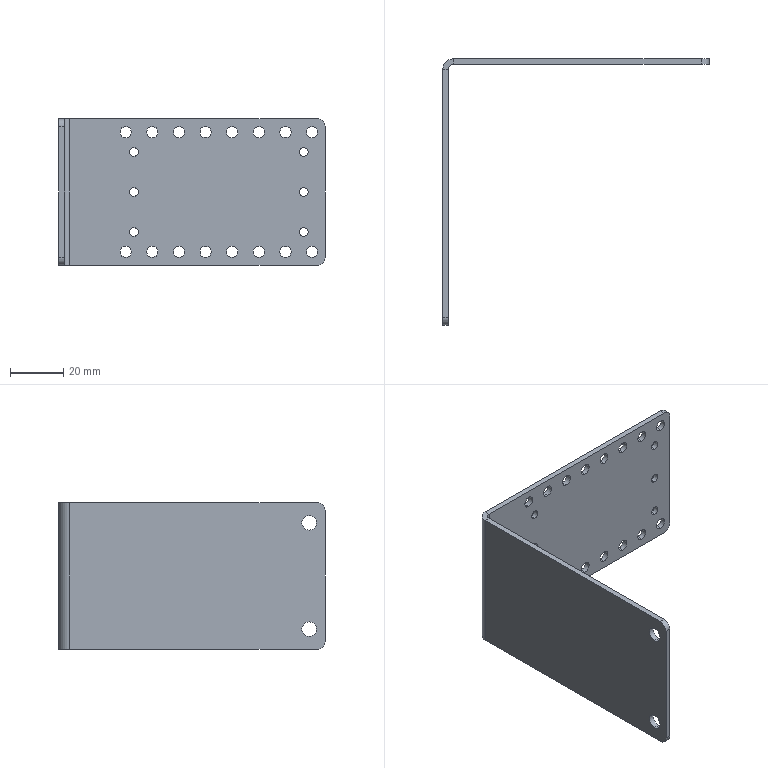Part | SolidWorks | features HoleWzd 3, Fillet 1, FlatPattern 1, SMBaseFlange 1, SheetMetal 1 | 1 solid | 66 faces | box 100 x 100 x 55 mm | volume 20982 mm3 | cylinder 54 | plane 12 | commonest cylinder face diameters 4.2 x32 3.3 x12 5.5 x4 6 x4 4 x1 8 x1